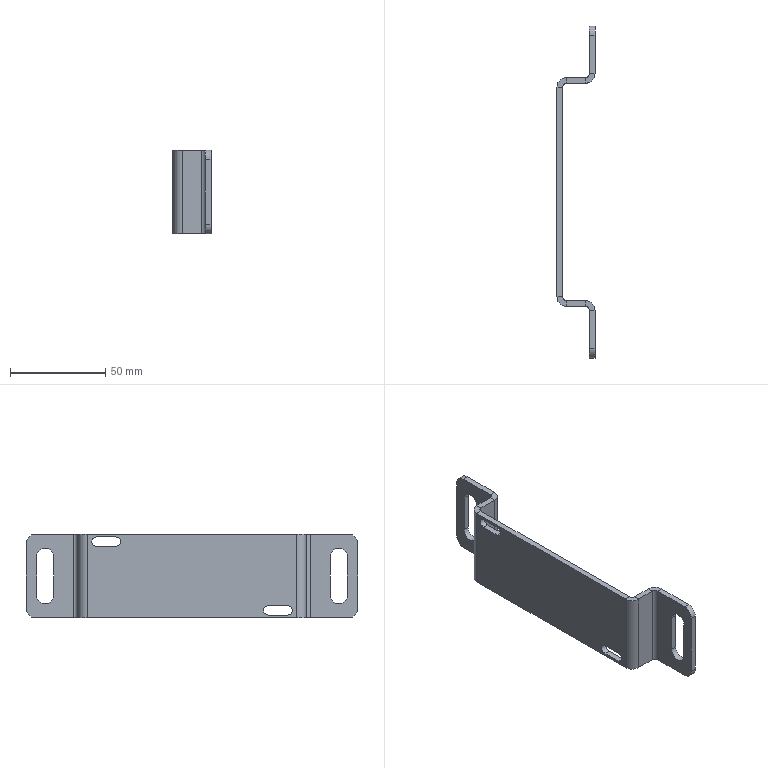Part | STEP file | 1 solid | 60 faces | box 20 x 174 x 44 mm | volume 24719 mm3 | plane 38 | cylinder 22 | commonest cylinder face diameters 10 x8 5 x6 4 x4 9 x4